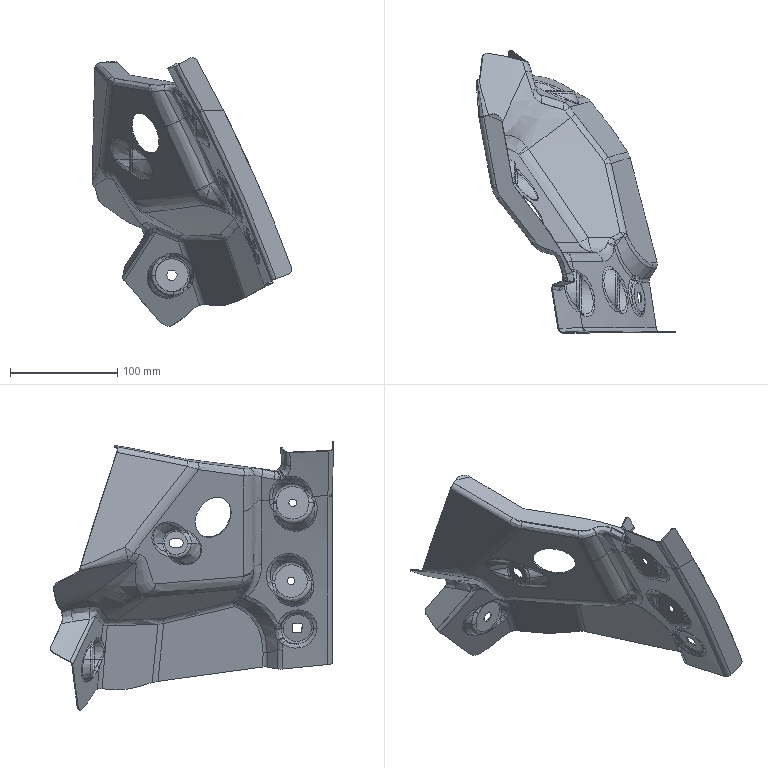Part | STEP file | FNA5401432 | 1 solid | 411 faces | box 186.294 x 264.478 x 250.717 mm | volume 73735 mm3 | spline 341 | cylinder 33 | plane 28 | sphere 6 | other 3 | commonest cylinder face diameters 2 x10 7 x4 40 x3 8 x2 10 x2 12 x1